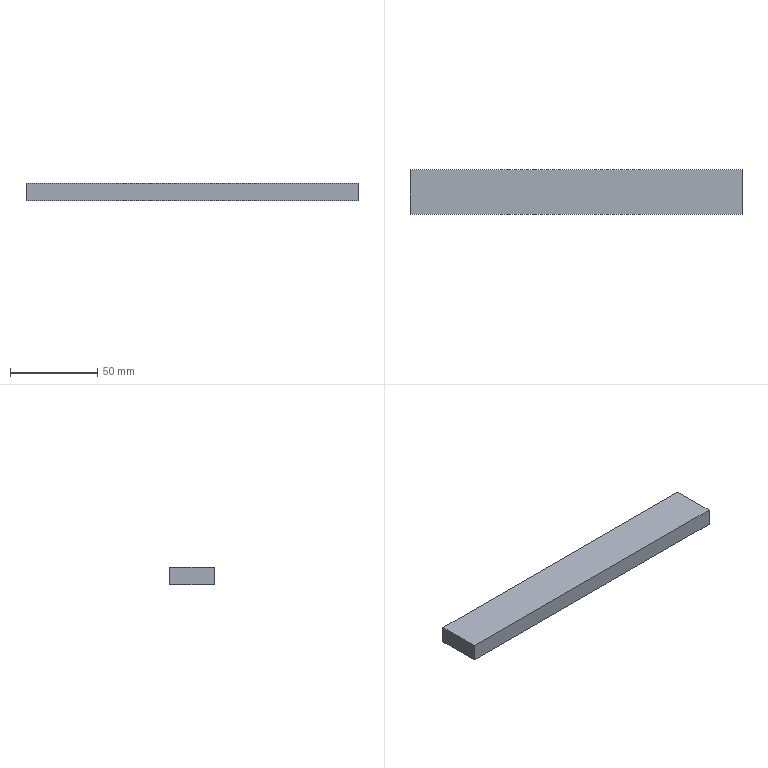Part | SolidWorks | features Extrusion 1 | 1 solid | 6 faces | box 190.5 x 25.4 x 10 mm | volume 48387 mm3 | plane 6
STEP:
#1=CARTESIAN_POINT('',(-95.25,12.7,-5.));
#2=VERTEX_POINT('',#1);
#3=CARTESIAN_POINT('',(-95.25,-12.7,-5.));
#4=VERTEX_POINT('',#3);
#5=CARTESIAN_POINT('',(-95.25,12.7,-5.));
#6=DIRECTION('',(0.,-1.,0.));
#7=VECTOR('',#6,1000.);
#8=LINE('',#5,#7);
#9=EDGE_CURVE('',#2,#4,#8,.T.);
#10=ORIENTED_EDGE('',*,*,#9,.T.);
#11=CARTESIAN_POINT('',(-95.25,-12.7,5.));
#12=VERTEX_POINT('',#11);
#13=CARTESIAN_POINT('',(-95.25,-12.7,5.));
#14=DIRECTION('',(0.,0.,-1.));
#15=VECTOR('',#14,1000.);
#16=LINE('',#13,#15);
#17=EDGE_CURVE('',#12,#4,#16,.T.);
#18=ORIENTED_EDGE('',*,*,#17,.F.);
#19=CARTESIAN_POINT('',(-95.25,12.7,5.));
#20=VERTEX_POINT('',#19);
#21=CARTESIAN_POINT('',(-95.25,12.7,5.));
#22=DIRECTION('',(0.,-1.,0.));
#23=VECTOR('',#22,1000.);
#24=LINE('',#21,#23);
#25=EDGE_CURVE('',#20,#12,#24,.T.);
#26=ORIENTED_EDGE('',*,*,#25,.F.);
#27=CARTESIAN_POINT('',(-95.25,12.7,5.));
#28=DIRECTION('',(0.,0.,-1.));
#29=VECTOR('',#28,1000.);
#30=LINE('',#27,#29);
#31=EDGE_CURVE('',#20,#2,#30,.T.);
#32=ORIENTED_EDGE('',*,*,#31,.T.);
#33=EDGE_LOOP('',(#10,#18,#26,#32));
#34=FACE_OUTER_BOUND('',#33,.T.);
#35=CARTESIAN_POINT('',(-95.25,12.7,5.));
#36=DIRECTION('',(1.,0.,0.));
#37=DIRECTION('',(0.,1.,0.));
#38=AXIS2_PLACEMENT_3D('',#35,#36,#37);
#39=PLANE('',#38);
#40=ADVANCED_FACE('',(#34),#39,.F.);
#41=CARTESIAN_POINT('',(95.25,-12.7,-5.));
#42=VERTEX_POINT('',#41);
#43=CARTESIAN_POINT('',(-95.25,-12.7,-5.));
#44=DIRECTION('',(1.,0.,0.));
#45=VECTOR('',#44,1000.);
#46=LINE('',#43,#45);
#47=EDGE_CURVE('',#4,#42,#46,.T.);
#48=ORIENTED_EDGE('',*,*,#47,.T.);
#49=CARTESIAN_POINT('',(95.25,-12.7,5.));
#50=VERTEX_POINT('',#49);
#51=CARTESIAN_POINT('',(95.25,-12.7,5.));
#52=DIRECTION('',(0.,0.,-1.));
#53=VECTOR('',#52,1000.);
#54=LINE('',#51,#53);
#55=EDGE_CURVE('',#50,#42,#54,.T.);
#56=ORIENTED_EDGE('',*,*,#55,.F.);
#57=CARTESIAN_POINT('',(-95.25,-12.7,5.));
#58=DIRECTION('',(1.,0.,0.));
#59=VECTOR('',#58,1000.);
#60=LINE('',#57,#59);
#61=EDGE_CURVE('',#12,#50,#60,.T.);
#62=ORIENTED_EDGE('',*,*,#61,.F.);
#63=ORIENTED_EDGE('',*,*,#17,.T.);
#64=EDGE_LOOP('',(#48,#56,#62,#63));
#65=FACE_OUTER_BOUND('',#64,.T.);
#66=CARTESIAN_POINT('',(-95.25,-12.7,5.));
#67=DIRECTION('',(0.,1.,0.));
#68=DIRECTION('',(-1.,0.,0.));
#69=AXIS2_PLACEMENT_3D('',#66,#67,#68);
#70=PLANE('',#69);
#71=ADVANCED_FACE('',(#65),#70,.F.);
#72=CARTESIAN_POINT('',(95.25,12.7,-5.));
#73=VERTEX_POINT('',#72);
#74=CARTESIAN_POINT('',(95.25,12.7,-5.));
#75=DIRECTION('',(0.,1.,0.));
#76=VECTOR('',#75,1000.);
#77=LINE('',#74,#76);
#78=EDGE_CURVE('',#42,#73,#77,.T.);
#79=ORIENTED_EDGE('',*,*,#78,.T.);
#80=CARTESIAN_POINT('',(95.25,12.7,5.));
#81=VERTEX_POINT('',#80);
#82=CARTESIAN_POINT('',(95.25,12.7,5.));
#83=DIRECTION('',(0.,0.,-1.));
#84=VECTOR('',#83,1000.);
#85=LINE('',#82,#84);
#86=EDGE_CURVE('',#81,#73,#85,.T.);
#87=ORIENTED_EDGE('',*,*,#86,.F.);
#88=CARTESIAN_POINT('',(95.25,12.7,5.));
#89=DIRECTION('',(0.,1.,0.));
#90=VECTOR('',#89,1000.);
#91=LINE('',#88,#90);
#92=EDGE_CURVE('',#50,#81,#91,.T.);
#93=ORIENTED_EDGE('',*,*,#92,.F.);
#94=ORIENTED_EDGE('',*,*,#55,.T.);
#95=EDGE_LOOP('',(#79,#87,#93,#94));
#96=FACE_OUTER_BOUND('',#95,.T.);
#97=CARTESIAN_POINT('',(95.25,12.7,5.));
#98=DIRECTION('',(-1.,0.,0.));
#99=DIRECTION('',(0.,-1.,0.));
#100=AXIS2_PLACEMENT_3D('',#97,#98,#99);
#101=PLANE('',#100);
#102=ADVANCED_FACE('',(#96),#101,.F.);
#103=CARTESIAN_POINT('',(-95.25,12.7,-5.));
#104=DIRECTION('',(-1.,0.,0.));
#105=VECTOR('',#104,1000.);
#106=LINE('',#103,#105);
#107=EDGE_CURVE('',#73,#2,#106,.T.);
#108=ORIENTED_EDGE('',*,*,#107,.T.);
#109=ORIENTED_EDGE('',*,*,#31,.F.);
#110=CARTESIAN_POINT('',(-95.25,12.7,5.));
#111=DIRECTION('',(-1.,0.,0.));
#112=VECTOR('',#111,1000.);
#113=LINE('',#110,#112);
#114=EDGE_CURVE('',#81,#20,#113,.T.);
#115=ORIENTED_EDGE('',*,*,#114,.F.);
#116=ORIENTED_EDGE('',*,*,#86,.T.);
#117=EDGE_LOOP('',(#108,#109,#115,#116));
#118=FACE_OUTER_BOUND('',#117,.T.);
#119=CARTESIAN_POINT('',(-95.25,12.7,5.));
#120=DIRECTION('',(0.,-1.,0.));
#121=DIRECTION('',(0.,0.,-1.));
#122=AXIS2_PLACEMENT_3D('',#119,#120,#121);
#123=PLANE('',#122);
#124=ADVANCED_FACE('',(#118),#123,.F.);
#125=ORIENTED_EDGE('',*,*,#25,.T.);
#126=ORIENTED_EDGE('',*,*,#61,.T.);
#127=ORIENTED_EDGE('',*,*,#92,.T.);
#128=ORIENTED_EDGE('',*,*,#114,.T.);
#129=EDGE_LOOP('',(#125,#126,#127,#128));
#130=FACE_OUTER_BOUND('',#129,.T.);
#131=CARTESIAN_POINT('',(0.,0.,5.));
#132=DIRECTION('',(0.,0.,1.));
#133=DIRECTION('',(1.,0.,0.));
#134=AXIS2_PLACEMENT_3D('',#131,#132,#133);
#135=PLANE('',#134);
#136=ADVANCED_FACE('',(#130),#135,.T.);
#137=ORIENTED_EDGE('',*,*,#9,.F.);
#138=ORIENTED_EDGE('',*,*,#107,.F.);
#139=ORIENTED_EDGE('',*,*,#78,.F.);
#140=ORIENTED_EDGE('',*,*,#47,.F.);
#141=EDGE_LOOP('',(#137,#138,#139,#140));
#142=FACE_OUTER_BOUND('',#141,.T.);
#143=CARTESIAN_POINT('',(0.,0.,-5.));
#144=DIRECTION('',(0.,0.,1.));
#145=DIRECTION('',(1.,0.,0.));
#146=AXIS2_PLACEMENT_3D('',#143,#144,#145);
#147=PLANE('',#146);
#148=ADVANCED_FACE('',(#142),#147,.F.);
#149=CLOSED_SHELL('',(#40,#71,#102,#124,#136,#148));
#150=MANIFOLD_SOLID_BREP('',#149);
#151=CARTESIAN_POINT('',(0.,0.,0.));
#152=DIRECTION('',(0.,0.,1.));
#153=DIRECTION('',(1.,0.,0.));
#154=AXIS2_PLACEMENT_3D('',#151,#152,#153);
#155=(LENGTH_UNIT()NAMED_UNIT(*)SI_UNIT(.MILLI.,.METRE.));
#156=UNCERTAINTY_MEASURE_WITH_UNIT(LENGTH_MEASURE(0.00001),#155,'','');
#157=(NAMED_UNIT(*)PLANE_ANGLE_UNIT()SI_UNIT($,.RADIAN.));
#158=(NAMED_UNIT(*)SI_UNIT($,.STERADIAN.)SOLID_ANGLE_UNIT());
#159=(GEOMETRIC_REPRESENTATION_CONTEXT(3)GLOBAL_UNCERTAINTY_ASSIGNED_CONTEXT((#156))GLOBAL_UNIT_ASSIGNED_CONTEXT((#155,#157,#158))REPRESENTATION_CONTEXT('',''));
#160=ADVANCED_BREP_SHAPE_REPRESENTATION('',(#150,#154),#159);